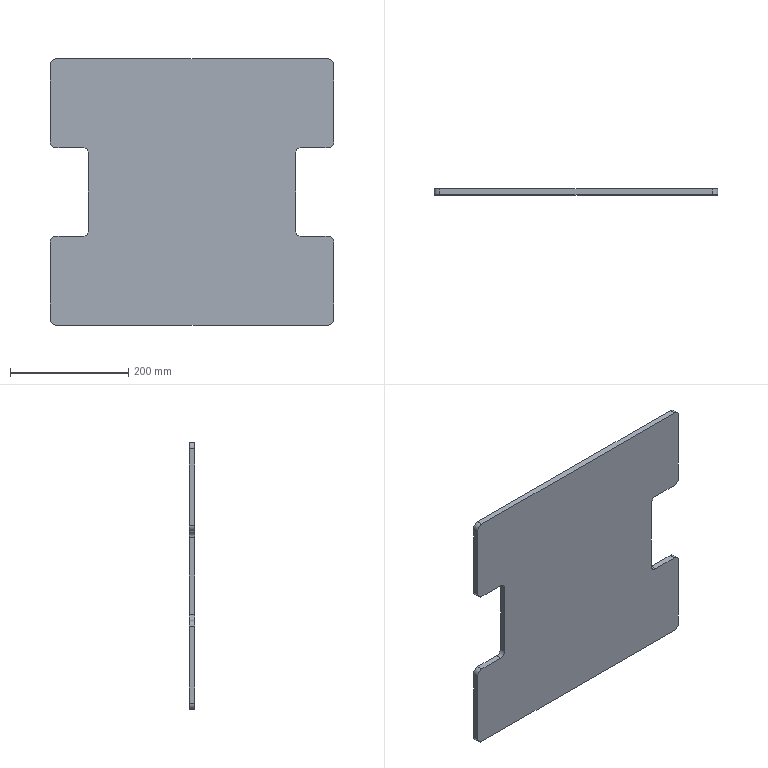Part | SolidWorks | features Fillet 2, ICE 2, Extrusion 1 | 1 solid | 26 faces | box 480 x 10 x 450 mm | volume 1964142 mm3 | plane 14 | cylinder 12 | commonest cylinder face diameters 20 x12
STEP:
#1=CARTESIAN_POINT('',(240.,0.,215.));
#2=VERTEX_POINT('',#1);
#3=CARTESIAN_POINT('',(240.,0.,85.));
#4=VERTEX_POINT('',#3);
#5=CARTESIAN_POINT('',(240.,0.,-325.));
#6=DIRECTION('',(0.,0.,-1.));
#7=VECTOR('',#6,1000.);
#8=LINE('',#5,#7);
#9=EDGE_CURVE('',#2,#4,#8,.T.);
#10=ORIENTED_EDGE('',*,*,#9,.T.);
#11=CARTESIAN_POINT('',(240.,10.,85.));
#12=VERTEX_POINT('',#11);
#13=CARTESIAN_POINT('',(240.,10.,85.));
#14=DIRECTION('',(0.,1.,0.));
#15=VECTOR('',#14,1000.);
#16=LINE('',#13,#15);
#17=EDGE_CURVE('',#4,#12,#16,.T.);
#18=ORIENTED_EDGE('',*,*,#17,.T.);
#19=CARTESIAN_POINT('',(240.,10.,215.));
#20=VERTEX_POINT('',#19);
#21=CARTESIAN_POINT('',(240.,10.,-325.));
#22=DIRECTION('',(0.,0.,-1.));
#23=VECTOR('',#22,1000.);
#24=LINE('',#21,#23);
#25=EDGE_CURVE('',#20,#12,#24,.T.);
#26=ORIENTED_EDGE('',*,*,#25,.F.);
#27=CARTESIAN_POINT('',(240.,10.,215.));
#28=DIRECTION('',(0.,-1.,0.));
#29=VECTOR('',#28,1000.);
#30=LINE('',#27,#29);
#31=EDGE_CURVE('',#20,#2,#30,.T.);
#32=ORIENTED_EDGE('',*,*,#31,.T.);
#33=EDGE_LOOP('',(#10,#18,#26,#32));
#34=FACE_OUTER_BOUND('',#33,.T.);
#35=CARTESIAN_POINT('',(240.,10.,-325.));
#36=DIRECTION('',(-1.,0.,0.));
#37=DIRECTION('',(0.,0.,1.));
#38=AXIS2_PLACEMENT_3D('',#35,#36,#37);
#39=PLANE('',#38);
#40=ADVANCED_FACE('',(#34),#39,.F.);
#41=CARTESIAN_POINT('',(-240.,10.,-215.));
#42=VERTEX_POINT('',#41);
#43=CARTESIAN_POINT('',(-240.,10.,-85.));
#44=VERTEX_POINT('',#43);
#45=CARTESIAN_POINT('',(-240.,10.,-325.));
#46=DIRECTION('',(0.,0.,1.));
#47=VECTOR('',#46,1000.);
#48=LINE('',#45,#47);
#49=EDGE_CURVE('',#42,#44,#48,.T.);
#50=ORIENTED_EDGE('',*,*,#49,.F.);
#51=CARTESIAN_POINT('',(-240.,0.,-215.));
#52=VERTEX_POINT('',#51);
#53=CARTESIAN_POINT('',(-240.,10.,-215.));
#54=DIRECTION('',(0.,-1.,0.));
#55=VECTOR('',#54,1000.);
#56=LINE('',#53,#55);
#57=EDGE_CURVE('',#42,#52,#56,.T.);
#58=ORIENTED_EDGE('',*,*,#57,.T.);
#59=CARTESIAN_POINT('',(-240.,0.,-85.));
#60=VERTEX_POINT('',#59);
#61=CARTESIAN_POINT('',(-240.,0.,-325.));
#62=DIRECTION('',(0.,0.,1.));
#63=VECTOR('',#62,1000.);
#64=LINE('',#61,#63);
#65=EDGE_CURVE('',#52,#60,#64,.T.);
#66=ORIENTED_EDGE('',*,*,#65,.T.);
#67=CARTESIAN_POINT('',(-240.,10.,-85.));
#68=DIRECTION('',(0.,1.,0.));
#69=VECTOR('',#68,1000.);
#70=LINE('',#67,#69);
#71=EDGE_CURVE('',#60,#44,#70,.T.);
#72=ORIENTED_EDGE('',*,*,#71,.T.);
#73=EDGE_LOOP('',(#50,#58,#66,#72));
#74=FACE_OUTER_BOUND('',#73,.T.);
#75=CARTESIAN_POINT('',(-240.,10.,-325.));
#76=DIRECTION('',(1.,0.,0.));
#77=DIRECTION('',(0.,0.,-1.));
#78=AXIS2_PLACEMENT_3D('',#75,#76,#77);
#79=PLANE('',#78);
#80=ADVANCED_FACE('',(#74),#79,.F.);
#81=CARTESIAN_POINT('',(-230.,10.,-225.));
#82=VERTEX_POINT('',#81);
#83=CARTESIAN_POINT('',(230.,10.,-225.));
#84=VERTEX_POINT('',#83);
#85=CARTESIAN_POINT('',(-281.378,10.,-225.));
#86=DIRECTION('',(1.,0.,0.));
#87=VECTOR('',#86,1000.);
#88=LINE('',#85,#87);
#89=EDGE_CURVE('',#82,#84,#88,.T.);
#90=ORIENTED_EDGE('',*,*,#89,.F.);
#91=CARTESIAN_POINT('',(-230.,10.,-215.));
#92=DIRECTION('',(0.,1.,0.));
#93=DIRECTION('',(0.,0.,1.));
#94=AXIS2_PLACEMENT_3D('',#91,#92,#93);
#95=CIRCLE('',#94,10.);
#96=EDGE_CURVE('',#82,#42,#95,.T.);
#97=ORIENTED_EDGE('',*,*,#96,.T.);
#98=ORIENTED_EDGE('',*,*,#49,.T.);
#99=CARTESIAN_POINT('',(-230.,10.,-75.));
#100=VERTEX_POINT('',#99);
#101=CARTESIAN_POINT('',(-230.,10.,-85.));
#102=DIRECTION('',(0.,1.,0.));
#103=DIRECTION('',(0.,0.,1.));
#104=AXIS2_PLACEMENT_3D('',#101,#102,#103);
#105=CIRCLE('',#104,10.);
#106=EDGE_CURVE('',#44,#100,#105,.T.);
#107=ORIENTED_EDGE('',*,*,#106,.T.);
#108=CARTESIAN_POINT('',(-185.,10.,-75.));
#109=VERTEX_POINT('',#108);
#110=CARTESIAN_POINT('',(-305.,10.,-75.));
#111=DIRECTION('',(1.,0.,0.));
#112=VECTOR('',#111,1000.);
#113=LINE('',#110,#112);
#114=EDGE_CURVE('',#100,#109,#113,.T.);
#115=ORIENTED_EDGE('',*,*,#114,.T.);
#116=CARTESIAN_POINT('',(-175.,10.,-65.));
#117=VERTEX_POINT('',#116);
#118=CARTESIAN_POINT('',(-185.,10.,-65.));
#119=DIRECTION('',(0.,-1.,0.));
#120=DIRECTION('',(0.,0.,1.));
#121=AXIS2_PLACEMENT_3D('',#118,#119,#120);
#122=CIRCLE('',#121,10.);
#123=EDGE_CURVE('',#109,#117,#122,.T.);
#124=ORIENTED_EDGE('',*,*,#123,.T.);
#125=CARTESIAN_POINT('',(-175.,10.,65.));
#126=VERTEX_POINT('',#125);
#127=CARTESIAN_POINT('',(-175.,10.,-75.));
#128=DIRECTION('',(0.,0.,1.));
#129=VECTOR('',#128,1000.);
#130=LINE('',#127,#129);
#131=EDGE_CURVE('',#117,#126,#130,.T.);
#132=ORIENTED_EDGE('',*,*,#131,.T.);
#133=CARTESIAN_POINT('',(-185.,10.,75.));
#134=VERTEX_POINT('',#133);
#135=CARTESIAN_POINT('',(-185.,10.,65.));
#136=DIRECTION('',(0.,-1.,0.));
#137=DIRECTION('',(0.,0.,1.));
#138=AXIS2_PLACEMENT_3D('',#135,#136,#137);
#139=CIRCLE('',#138,10.);
#140=EDGE_CURVE('',#126,#134,#139,.T.);
#141=ORIENTED_EDGE('',*,*,#140,.T.);
#142=CARTESIAN_POINT('',(-230.,10.,75.));
#143=VERTEX_POINT('',#142);
#144=CARTESIAN_POINT('',(-305.,10.,75.));
#145=DIRECTION('',(1.,0.,0.));
#146=VECTOR('',#145,1000.);
#147=LINE('',#144,#146);
#148=EDGE_CURVE('',#143,#134,#147,.T.);
#149=ORIENTED_EDGE('',*,*,#148,.F.);
#150=CARTESIAN_POINT('',(-240.,10.,85.));
#151=VERTEX_POINT('',#150);
#152=CARTESIAN_POINT('',(-230.,10.,85.));
#153=DIRECTION('',(0.,1.,0.));
#154=DIRECTION('',(0.,0.,1.));
#155=AXIS2_PLACEMENT_3D('',#152,#153,#154);
#156=CIRCLE('',#155,10.);
#157=EDGE_CURVE('',#143,#151,#156,.T.);
#158=ORIENTED_EDGE('',*,*,#157,.T.);
#159=CARTESIAN_POINT('',(-240.,10.,215.));
#160=VERTEX_POINT('',#159);
#161=CARTESIAN_POINT('',(-240.,10.,-325.));
#162=DIRECTION('',(0.,0.,1.));
#163=VECTOR('',#162,1000.);
#164=LINE('',#161,#163);
#165=EDGE_CURVE('',#151,#160,#164,.T.);
#166=ORIENTED_EDGE('',*,*,#165,.T.);
#167=CARTESIAN_POINT('',(-230.,10.,225.));
#168=VERTEX_POINT('',#167);
#169=CARTESIAN_POINT('',(-230.,10.,215.));
#170=DIRECTION('',(0.,1.,0.));
#171=DIRECTION('',(0.,0.,1.));
#172=AXIS2_PLACEMENT_3D('',#169,#170,#171);
#173=CIRCLE('',#172,10.);
#174=EDGE_CURVE('',#160,#168,#173,.T.);
#175=ORIENTED_EDGE('',*,*,#174,.T.);
#176=CARTESIAN_POINT('',(230.,10.,225.));
#177=VERTEX_POINT('',#176);
#178=CARTESIAN_POINT('',(-281.378,10.,225.));
#179=DIRECTION('',(-1.,0.,0.));
#180=VECTOR('',#179,1000.);
#181=LINE('',#178,#180);
#182=EDGE_CURVE('',#177,#168,#181,.T.);
#183=ORIENTED_EDGE('',*,*,#182,.F.);
#184=CARTESIAN_POINT('',(230.,10.,215.));
#185=DIRECTION('',(0.,1.,0.));
#186=DIRECTION('',(0.,0.,1.));
#187=AXIS2_PLACEMENT_3D('',#184,#185,#186);
#188=CIRCLE('',#187,10.);
#189=EDGE_CURVE('',#177,#20,#188,.T.);
#190=ORIENTED_EDGE('',*,*,#189,.T.);
#191=ORIENTED_EDGE('',*,*,#25,.T.);
#192=CARTESIAN_POINT('',(230.,10.,75.));
#193=VERTEX_POINT('',#192);
#194=CARTESIAN_POINT('',(230.,10.,85.));
#195=DIRECTION('',(0.,1.,0.));
#196=DIRECTION('',(0.,0.,1.));
#197=AXIS2_PLACEMENT_3D('',#194,#195,#196);
#198=CIRCLE('',#197,10.);
#199=EDGE_CURVE('',#12,#193,#198,.T.);
#200=ORIENTED_EDGE('',*,*,#199,.T.);
#201=CARTESIAN_POINT('',(185.,10.,75.));
#202=VERTEX_POINT('',#201);
#203=CARTESIAN_POINT('',(305.,10.,75.));
#204=DIRECTION('',(-1.,0.,0.));
#205=VECTOR('',#204,1000.);
#206=LINE('',#203,#205);
#207=EDGE_CURVE('',#193,#202,#206,.T.);
#208=ORIENTED_EDGE('',*,*,#207,.T.);
#209=CARTESIAN_POINT('',(175.,10.,65.));
#210=VERTEX_POINT('',#209);
#211=CARTESIAN_POINT('',(185.,10.,65.));
#212=DIRECTION('',(0.,-1.,0.));
#213=DIRECTION('',(0.,0.,1.));
#214=AXIS2_PLACEMENT_3D('',#211,#212,#213);
#215=CIRCLE('',#214,10.);
#216=EDGE_CURVE('',#202,#210,#215,.T.);
#217=ORIENTED_EDGE('',*,*,#216,.T.);
#218=CARTESIAN_POINT('',(175.,10.,-65.));
#219=VERTEX_POINT('',#218);
#220=CARTESIAN_POINT('',(175.,10.,-75.));
#221=DIRECTION('',(0.,0.,1.));
#222=VECTOR('',#221,1000.);
#223=LINE('',#220,#222);
#224=EDGE_CURVE('',#219,#210,#223,.T.);
#225=ORIENTED_EDGE('',*,*,#224,.F.);
#226=CARTESIAN_POINT('',(185.,10.,-75.));
#227=VERTEX_POINT('',#226);
#228=CARTESIAN_POINT('',(185.,10.,-65.));
#229=DIRECTION('',(0.,-1.,0.));
#230=DIRECTION('',(0.,0.,1.));
#231=AXIS2_PLACEMENT_3D('',#228,#229,#230);
#232=CIRCLE('',#231,10.);
#233=EDGE_CURVE('',#219,#227,#232,.T.);
#234=ORIENTED_EDGE('',*,*,#233,.T.);
#235=CARTESIAN_POINT('',(230.,10.,-75.));
#236=VERTEX_POINT('',#235);
#237=CARTESIAN_POINT('',(305.,10.,-75.));
#238=DIRECTION('',(-1.,0.,0.));
#239=VECTOR('',#238,1000.);
#240=LINE('',#237,#239);
#241=EDGE_CURVE('',#236,#227,#240,.T.);
#242=ORIENTED_EDGE('',*,*,#241,.F.);
#243=CARTESIAN_POINT('',(240.,10.,-85.));
#244=VERTEX_POINT('',#243);
#245=CARTESIAN_POINT('',(230.,10.,-85.));
#246=DIRECTION('',(0.,1.,0.));
#247=DIRECTION('',(0.,0.,1.));
#248=AXIS2_PLACEMENT_3D('',#245,#246,#247);
#249=CIRCLE('',#248,10.);
#250=EDGE_CURVE('',#236,#244,#249,.T.);
#251=ORIENTED_EDGE('',*,*,#250,.T.);
#252=CARTESIAN_POINT('',(240.,10.,-215.));
#253=VERTEX_POINT('',#252);
#254=CARTESIAN_POINT('',(240.,10.,-325.));
#255=DIRECTION('',(0.,0.,-1.));
#256=VECTOR('',#255,1000.);
#257=LINE('',#254,#256);
#258=EDGE_CURVE('',#244,#253,#257,.T.);
#259=ORIENTED_EDGE('',*,*,#258,.T.);
#260=CARTESIAN_POINT('',(230.,10.,-215.));
#261=DIRECTION('',(0.,1.,0.));
#262=DIRECTION('',(0.,0.,1.));
#263=AXIS2_PLACEMENT_3D('',#260,#261,#262);
#264=CIRCLE('',#263,10.);
#265=EDGE_CURVE('',#253,#84,#264,.T.);
#266=ORIENTED_EDGE('',*,*,#265,.T.);
#267=EDGE_LOOP('',(#90,#97,#98,#107,#115,#124,#132,#141,#149,#158,#166,#175,#183,#190,#191,#200,#208,#217,#225,#234,#242,#251,#259,#266));
#268=FACE_OUTER_BOUND('',#267,.T.);
#269=CARTESIAN_POINT('',(0.,10.,0.));
#270=DIRECTION('',(0.,1.,0.));
#271=DIRECTION('',(0.,0.,1.));
#272=AXIS2_PLACEMENT_3D('',#269,#270,#271);
#273=PLANE('',#272);
#274=ADVANCED_FACE('',(#268),#273,.T.);
#275=ORIENTED_EDGE('',*,*,#65,.F.);
#276=CARTESIAN_POINT('',(-230.,0.,-225.));
#277=VERTEX_POINT('',#276);
#278=CARTESIAN_POINT('',(-230.,0.,-215.));
#279=DIRECTION('',(0.,-1.,0.));
#280=DIRECTION('',(0.,0.,1.));
#281=AXIS2_PLACEMENT_3D('',#278,#279,#280);
#282=CIRCLE('',#281,10.);
#283=EDGE_CURVE('',#52,#277,#282,.T.);
#284=ORIENTED_EDGE('',*,*,#283,.T.);
#285=CARTESIAN_POINT('',(230.,0.,-225.));
#286=VERTEX_POINT('',#285);
#287=CARTESIAN_POINT('',(-281.378,0.,-225.));
#288=DIRECTION('',(1.,0.,0.));
#289=VECTOR('',#288,1000.);
#290=LINE('',#287,#289);
#291=EDGE_CURVE('',#277,#286,#290,.T.);
#292=ORIENTED_EDGE('',*,*,#291,.T.);
#293=CARTESIAN_POINT('',(240.,0.,-215.));
#294=VERTEX_POINT('',#293);
#295=CARTESIAN_POINT('',(230.,0.,-215.));
#296=DIRECTION('',(0.,-1.,0.));
#297=DIRECTION('',(0.,0.,1.));
#298=AXIS2_PLACEMENT_3D('',#295,#296,#297);
#299=CIRCLE('',#298,10.);
#300=EDGE_CURVE('',#286,#294,#299,.T.);
#301=ORIENTED_EDGE('',*,*,#300,.T.);
#302=CARTESIAN_POINT('',(240.,0.,-85.));
#303=VERTEX_POINT('',#302);
#304=CARTESIAN_POINT('',(240.,0.,-325.));
#305=DIRECTION('',(0.,0.,-1.));
#306=VECTOR('',#305,1000.);
#307=LINE('',#304,#306);
#308=EDGE_CURVE('',#303,#294,#307,.T.);
#309=ORIENTED_EDGE('',*,*,#308,.F.);
#310=CARTESIAN_POINT('',(230.,0.,-75.));
#311=VERTEX_POINT('',#310);
#312=CARTESIAN_POINT('',(230.,0.,-85.));
#313=DIRECTION('',(0.,-1.,0.));
#314=DIRECTION('',(0.,0.,1.));
#315=AXIS2_PLACEMENT_3D('',#312,#313,#314);
#316=CIRCLE('',#315,10.);
#317=EDGE_CURVE('',#303,#311,#316,.T.);
#318=ORIENTED_EDGE('',*,*,#317,.T.);
#319=CARTESIAN_POINT('',(185.,0.,-75.));
#320=VERTEX_POINT('',#319);
#321=CARTESIAN_POINT('',(0.,0.,-75.));
#322=DIRECTION('',(-1.,0.,0.));
#323=VECTOR('',#322,1000.);
#324=LINE('',#321,#323);
#325=EDGE_CURVE('',#311,#320,#324,.T.);
#326=ORIENTED_EDGE('',*,*,#325,.T.);
#327=CARTESIAN_POINT('',(175.,0.,-65.));
#328=VERTEX_POINT('',#327);
#329=CARTESIAN_POINT('',(185.,0.,-65.));
#330=DIRECTION('',(0.,1.,0.));
#331=DIRECTION('',(0.,0.,1.));
#332=AXIS2_PLACEMENT_3D('',#329,#330,#331);
#333=CIRCLE('',#332,10.);
#334=EDGE_CURVE('',#320,#328,#333,.T.);
#335=ORIENTED_EDGE('',*,*,#334,.T.);
#336=CARTESIAN_POINT('',(175.,0.,65.));
#337=VERTEX_POINT('',#336);
#338=CARTESIAN_POINT('',(175.,0.,-75.));
#339=DIRECTION('',(0.,0.,1.));
#340=VECTOR('',#339,1000.);
#341=LINE('',#338,#340);
#342=EDGE_CURVE('',#328,#337,#341,.T.);
#343=ORIENTED_EDGE('',*,*,#342,.T.);
#344=CARTESIAN_POINT('',(185.,0.,75.));
#345=VERTEX_POINT('',#344);
#346=CARTESIAN_POINT('',(185.,0.,65.));
#347=DIRECTION('',(0.,1.,0.));
#348=DIRECTION('',(0.,0.,1.));
#349=AXIS2_PLACEMENT_3D('',#346,#347,#348);
#350=CIRCLE('',#349,10.);
#351=EDGE_CURVE('',#337,#345,#350,.T.);
#352=ORIENTED_EDGE('',*,*,#351,.T.);
#353=CARTESIAN_POINT('',(230.,0.,75.));
#354=VERTEX_POINT('',#353);
#355=CARTESIAN_POINT('',(0.,0.,75.));
#356=DIRECTION('',(-1.,0.,0.));
#357=VECTOR('',#356,1000.);
#358=LINE('',#355,#357);
#359=EDGE_CURVE('',#354,#345,#358,.T.);
#360=ORIENTED_EDGE('',*,*,#359,.F.);
#361=CARTESIAN_POINT('',(230.,0.,85.));
#362=DIRECTION('',(0.,-1.,0.));
#363=DIRECTION('',(0.,0.,1.));
#364=AXIS2_PLACEMENT_3D('',#361,#362,#363);
#365=CIRCLE('',#364,10.);
#366=EDGE_CURVE('',#354,#4,#365,.T.);
#367=ORIENTED_EDGE('',*,*,#366,.T.);
#368=ORIENTED_EDGE('',*,*,#9,.F.);
#369=CARTESIAN_POINT('',(230.,0.,225.));
#370=VERTEX_POINT('',#369);
#371=CARTESIAN_POINT('',(230.,0.,215.));
#372=DIRECTION('',(0.,-1.,0.));
#373=DIRECTION('',(0.,0.,1.));
#374=AXIS2_PLACEMENT_3D('',#371,#372,#373);
#375=CIRCLE('',#374,10.);
#376=EDGE_CURVE('',#2,#370,#375,.T.);
#377=ORIENTED_EDGE('',*,*,#376,.T.);
#378=CARTESIAN_POINT('',(-230.,0.,225.));
#379=VERTEX_POINT('',#378);
#380=CARTESIAN_POINT('',(-281.378,0.,225.));
#381=DIRECTION('',(-1.,0.,0.));
#382=VECTOR('',#381,1000.);
#383=LINE('',#380,#382);
#384=EDGE_CURVE('',#370,#379,#383,.T.);
#385=ORIENTED_EDGE('',*,*,#384,.T.);
#386=CARTESIAN_POINT('',(-240.,0.,215.));
#387=VERTEX_POINT('',#386);
#388=CARTESIAN_POINT('',(-230.,0.,215.));
#389=DIRECTION('',(0.,-1.,0.));
#390=DIRECTION('',(0.,0.,1.));
#391=AXIS2_PLACEMENT_3D('',#388,#389,#390);
#392=CIRCLE('',#391,10.);
#393=EDGE_CURVE('',#379,#387,#392,.T.);
#394=ORIENTED_EDGE('',*,*,#393,.T.);
#395=CARTESIAN_POINT('',(-240.,0.,85.));
#396=VERTEX_POINT('',#395);
#397=CARTESIAN_POINT('',(-240.,0.,-325.));
#398=DIRECTION('',(0.,0.,1.));
#399=VECTOR('',#398,1000.);
#400=LINE('',#397,#399);
#401=EDGE_CURVE('',#396,#387,#400,.T.);
#402=ORIENTED_EDGE('',*,*,#401,.F.);
#403=CARTESIAN_POINT('',(-230.,0.,75.));
#404=VERTEX_POINT('',#403);
#405=CARTESIAN_POINT('',(-230.,0.,85.));
#406=DIRECTION('',(0.,-1.,0.));
#407=DIRECTION('',(0.,0.,1.));
#408=AXIS2_PLACEMENT_3D('',#405,#406,#407);
#409=CIRCLE('',#408,10.);
#410=EDGE_CURVE('',#396,#404,#409,.T.);
#411=ORIENTED_EDGE('',*,*,#410,.T.);
#412=CARTESIAN_POINT('',(-185.,0.,75.));
#413=VERTEX_POINT('',#412);
#414=CARTESIAN_POINT('',(0.,0.,75.));
#415=DIRECTION('',(1.,0.,0.));
#416=VECTOR('',#415,1000.);
#417=LINE('',#414,#416);
#418=EDGE_CURVE('',#404,#413,#417,.T.);
#419=ORIENTED_EDGE('',*,*,#418,.T.);
#420=CARTESIAN_POINT('',(-175.,0.,65.));
#421=VERTEX_POINT('',#420);
#422=CARTESIAN_POINT('',(-185.,0.,65.));
#423=DIRECTION('',(0.,1.,0.));
#424=DIRECTION('',(0.,0.,1.));
#425=AXIS2_PLACEMENT_3D('',#422,#423,#424);
#426=CIRCLE('',#425,10.);
#427=EDGE_CURVE('',#413,#421,#426,.T.);
#428=ORIENTED_EDGE('',*,*,#427,.T.);
#429=CARTESIAN_POINT('',(-175.,0.,-65.));
#430=VERTEX_POINT('',#429);
#431=CARTESIAN_POINT('',(-175.,0.,-75.));
#432=DIRECTION('',(0.,0.,1.));
#433=VECTOR('',#432,1000.);
#434=LINE('',#431,#433);
#435=EDGE_CURVE('',#430,#421,#434,.T.);
#436=ORIENTED_EDGE('',*,*,#435,.F.);
#437=CARTESIAN_POINT('',(-185.,0.,-75.));
#438=VERTEX_POINT('',#437);
#439=CARTESIAN_POINT('',(-185.,0.,-65.));
#440=DIRECTION('',(0.,1.,0.));
#441=DIRECTION('',(0.,0.,1.));
#442=AXIS2_PLACEMENT_3D('',#439,#440,#441);
#443=CIRCLE('',#442,10.);
#444=EDGE_CURVE('',#430,#438,#443,.T.);
#445=ORIENTED_EDGE('',*,*,#444,.T.);
#446=CARTESIAN_POINT('',(-230.,0.,-75.));
#447=VERTEX_POINT('',#446);
#448=CARTESIAN_POINT('',(0.,0.,-75.));
#449=DIRECTION('',(1.,0.,0.));
#450=VECTOR('',#449,1000.);
#451=LINE('',#448,#450);
#452=EDGE_CURVE('',#447,#438,#451,.T.);
#453=ORIENTED_EDGE('',*,*,#452,.F.);
#454=CARTESIAN_POINT('',(-230.,0.,-85.));
#455=DIRECTION('',(0.,-1.,0.));
#456=DIRECTION('',(0.,0.,1.));
#457=AXIS2_PLACEMENT_3D('',#454,#455,#456);
#458=CIRCLE('',#457,10.);
#459=EDGE_CURVE('',#447,#60,#458,.T.);
#460=ORIENTED_EDGE('',*,*,#459,.T.);
#461=EDGE_LOOP('',(#275,#284,#292,#301,#309,#318,#326,#335,#343,#352,#360,#367,#368,#377,#385,#394,#402,#411,#419,#428,#436,#445,#453,#460));
#462=FACE_OUTER_BOUND('',#461,.T.);
#463=CARTESIAN_POINT('',(0.,0.,0.));
#464=DIRECTION('',(0.,1.,0.));
#465=DIRECTION('',(0.,0.,1.));
#466=AXIS2_PLACEMENT_3D('',#463,#464,#465);
#467=PLANE('',#466);
#468=ADVANCED_FACE('',(#462),#467,.F.);
#469=ORIENTED_EDGE('',*,*,#308,.T.);
#470=CARTESIAN_POINT('',(240.,10.,-215.));
#471=DIRECTION('',(0.,1.,0.));
#472=VECTOR('',#471,1000.);
#473=LINE('',#470,#472);
#474=EDGE_CURVE('',#294,#253,#473,.T.);
#475=ORIENTED_EDGE('',*,*,#474,.T.);
#476=ORIENTED_EDGE('',*,*,#258,.F.);
#477=CARTESIAN_POINT('',(240.,10.,-85.));
#478=DIRECTION('',(0.,-1.,0.));
#479=VECTOR('',#478,1000.);
#480=LINE('',#477,#479);
#481=EDGE_CURVE('',#244,#303,#480,.T.);
#482=ORIENTED_EDGE('',*,*,#481,.T.);
#483=EDGE_LOOP('',(#469,#475,#476,#482));
#484=FACE_OUTER_BOUND('',#483,.T.);
#485=CARTESIAN_POINT('',(240.,10.,-325.));
#486=DIRECTION('',(-1.,0.,0.));
#487=DIRECTION('',(0.,0.,1.));
#488=AXIS2_PLACEMENT_3D('',#485,#486,#487);
#489=PLANE('',#488);
#490=ADVANCED_FACE('',(#484),#489,.F.);
#491=ORIENTED_EDGE('',*,*,#401,.T.);
#492=CARTESIAN_POINT('',(-240.,10.,215.));
#493=DIRECTION('',(0.,1.,0.));
#494=VECTOR('',#493,1000.);
#495=LINE('',#492,#494);
#496=EDGE_CURVE('',#387,#160,#495,.T.);
#497=ORIENTED_EDGE('',*,*,#496,.T.);
#498=ORIENTED_EDGE('',*,*,#165,.F.);
#499=CARTESIAN_POINT('',(-240.,10.,85.));
#500=DIRECTION('',(0.,-1.,0.));
#501=VECTOR('',#500,1000.);
#502=LINE('',#499,#501);
#503=EDGE_CURVE('',#151,#396,#502,.T.);
#504=ORIENTED_EDGE('',*,*,#503,.T.);
#505=EDGE_LOOP('',(#491,#497,#498,#504));
#506=FACE_OUTER_BOUND('',#505,.T.);
#507=CARTESIAN_POINT('',(-240.,10.,-325.));
#508=DIRECTION('',(1.,0.,0.));
#509=DIRECTION('',(0.,0.,-1.));
#510=AXIS2_PLACEMENT_3D('',#507,#508,#509);
#511=PLANE('',#510);
#512=ADVANCED_FACE('',(#506),#511,.F.);
#513=ORIENTED_EDGE('',*,*,#325,.F.);
#514=CARTESIAN_POINT('',(230.,0.,-75.));
#515=DIRECTION('',(0.,1.,0.));
#516=VECTOR('',#515,1000.);
#517=LINE('',#514,#516);
#518=EDGE_CURVE('',#311,#236,#517,.T.);
#519=ORIENTED_EDGE('',*,*,#518,.T.);
#520=ORIENTED_EDGE('',*,*,#241,.T.);
#521=CARTESIAN_POINT('',(185.,0.,-75.));
#522=DIRECTION('',(0.,-1.,0.));
#523=VECTOR('',#522,1000.);
#524=LINE('',#521,#523);
#525=EDGE_CURVE('',#227,#320,#524,.T.);
#526=ORIENTED_EDGE('',*,*,#525,.T.);
#527=EDGE_LOOP('',(#513,#519,#520,#526));
#528=FACE_OUTER_BOUND('',#527,.T.);
#529=CARTESIAN_POINT('',(305.,0.,-75.));
#530=DIRECTION('',(0.,0.,-1.));
#531=DIRECTION('',(-1.,0.,0.));
#532=AXIS2_PLACEMENT_3D('',#529,#530,#531);
#533=PLANE('',#532);
#534=ADVANCED_FACE('',(#528),#533,.F.);
#535=ORIENTED_EDGE('',*,*,#359,.T.);
#536=CARTESIAN_POINT('',(185.,0.,75.));
#537=DIRECTION('',(0.,1.,0.));
#538=VECTOR('',#537,1000.);
#539=LINE('',#536,#538);
#540=EDGE_CURVE('',#345,#202,#539,.T.);
#541=ORIENTED_EDGE('',*,*,#540,.T.);
#542=ORIENTED_EDGE('',*,*,#207,.F.);
#543=CARTESIAN_POINT('',(230.,0.,75.));
#544=DIRECTION('',(0.,-1.,0.));
#545=VECTOR('',#544,1000.);
#546=LINE('',#543,#545);
#547=EDGE_CURVE('',#193,#354,#546,.T.);
#548=ORIENTED_EDGE('',*,*,#547,.T.);
#549=EDGE_LOOP('',(#535,#541,#542,#548));
#550=FACE_OUTER_BOUND('',#549,.T.);
#551=CARTESIAN_POINT('',(305.,0.,75.));
#552=DIRECTION('',(0.,0.,-1.));
#553=DIRECTION('',(-1.,0.,0.));
#554=AXIS2_PLACEMENT_3D('',#551,#552,#553);
#555=PLANE('',#554);
#556=ADVANCED_FACE('',(#550),#555,.T.);
#557=ORIENTED_EDGE('',*,*,#342,.F.);
#558=CARTESIAN_POINT('',(175.,10.,-65.));
#559=DIRECTION('',(0.,1.,0.));
#560=VECTOR('',#559,1000.);
#561=LINE('',#558,#560);
#562=EDGE_CURVE('',#328,#219,#561,.T.);
#563=ORIENTED_EDGE('',*,*,#562,.T.);
#564=ORIENTED_EDGE('',*,*,#224,.T.);
#565=CARTESIAN_POINT('',(175.,0.,65.));
#566=DIRECTION('',(0.,-1.,0.));
#567=VECTOR('',#566,1000.);
#568=LINE('',#565,#567);
#569=EDGE_CURVE('',#210,#337,#568,.T.);
#570=ORIENTED_EDGE('',*,*,#569,.T.);
#571=EDGE_LOOP('',(#557,#563,#564,#570));
#572=FACE_OUTER_BOUND('',#571,.T.);
#573=CARTESIAN_POINT('',(175.,0.,-75.));
#574=DIRECTION('',(-1.,0.,0.));
#575=DIRECTION('',(0.,0.,1.));
#576=AXIS2_PLACEMENT_3D('',#573,#574,#575);
#577=PLANE('',#576);
#578=ADVANCED_FACE('',(#572),#577,.F.);
#579=ORIENTED_EDGE('',*,*,#452,.T.);
#580=CARTESIAN_POINT('',(-185.,10.,-75.));
#581=DIRECTION('',(0.,1.,0.));
#582=VECTOR('',#581,1000.);
#583=LINE('',#580,#582);
#584=EDGE_CURVE('',#438,#109,#583,.T.);
#585=ORIENTED_EDGE('',*,*,#584,.T.);
#586=ORIENTED_EDGE('',*,*,#114,.F.);
#587=CARTESIAN_POINT('',(-230.,0.,-75.));
#588=DIRECTION('',(0.,-1.,0.));
#589=VECTOR('',#588,1000.);
#590=LINE('',#587,#589);
#591=EDGE_CURVE('',#100,#447,#590,.T.);
#592=ORIENTED_EDGE('',*,*,#591,.T.);
#593=EDGE_LOOP('',(#579,#585,#586,#592));
#594=FACE_OUTER_BOUND('',#593,.T.);
#595=CARTESIAN_POINT('',(-305.,0.,-75.));
#596=DIRECTION('',(0.,0.,1.));
#597=DIRECTION('',(1.,0.,0.));
#598=AXIS2_PLACEMENT_3D('',#595,#596,#597);
#599=PLANE('',#598);
#600=ADVANCED_FACE('',(#594),#599,.T.);
#601=ORIENTED_EDGE('',*,*,#418,.F.);
#602=CARTESIAN_POINT('',(-230.,0.,75.));
#603=DIRECTION('',(0.,1.,0.));
#604=VECTOR('',#603,1000.);
#605=LINE('',#602,#604);
#606=EDGE_CURVE('',#404,#143,#605,.T.);
#607=ORIENTED_EDGE('',*,*,#606,.T.);
#608=ORIENTED_EDGE('',*,*,#148,.T.);
#609=CARTESIAN_POINT('',(-185.,0.,75.));
#610=DIRECTION('',(0.,-1.,0.));
#611=VECTOR('',#610,1000.);
#612=LINE('',#609,#611);
#613=EDGE_CURVE('',#134,#413,#612,.T.);
#614=ORIENTED_EDGE('',*,*,#613,.T.);
#615=EDGE_LOOP('',(#601,#607,#608,#614));
#616=FACE_OUTER_BOUND('',#615,.T.);
#617=CARTESIAN_POINT('',(-305.,0.,75.));
#618=DIRECTION('',(0.,0.,1.));
#619=DIRECTION('',(1.,0.,0.));
#620=AXIS2_PLACEMENT_3D('',#617,#618,#619);
#621=PLANE('',#620);
#622=ADVANCED_FACE('',(#616),#621,.F.);
#623=ORIENTED_EDGE('',*,*,#435,.T.);
#624=CARTESIAN_POINT('',(-175.,0.,65.));
#625=DIRECTION('',(0.,1.,0.));
#626=VECTOR('',#625,1000.);
#627=LINE('',#624,#626);
#628=EDGE_CURVE('',#421,#126,#627,.T.);
#629=ORIENTED_EDGE('',*,*,#628,.T.);
#630=ORIENTED_EDGE('',*,*,#131,.F.);
#631=CARTESIAN_POINT('',(-175.,0.,-65.));
#632=DIRECTION('',(0.,-1.,0.));
#633=VECTOR('',#632,1000.);
#634=LINE('',#631,#633);
#635=EDGE_CURVE('',#117,#430,#634,.T.);
#636=ORIENTED_EDGE('',*,*,#635,.T.);
#637=EDGE_LOOP('',(#623,#629,#630,#636));
#638=FACE_OUTER_BOUND('',#637,.T.);
#639=CARTESIAN_POINT('',(-175.,0.,-75.));
#640=DIRECTION('',(-1.,0.,0.));
#641=DIRECTION('',(0.,0.,1.));
#642=AXIS2_PLACEMENT_3D('',#639,#640,#641);
#643=PLANE('',#642);
#644=ADVANCED_FACE('',(#638),#643,.T.);
#645=ORIENTED_EDGE('',*,*,#384,.F.);
#646=CARTESIAN_POINT('',(230.,0.,225.));
#647=DIRECTION('',(0.,1.,0.));
#648=VECTOR('',#647,1000.);
#649=LINE('',#646,#648);
#650=EDGE_CURVE('',#370,#177,#649,.T.);
#651=ORIENTED_EDGE('',*,*,#650,.T.);
#652=ORIENTED_EDGE('',*,*,#182,.T.);
#653=CARTESIAN_POINT('',(-230.,0.,225.));
#654=DIRECTION('',(0.,-1.,0.));
#655=VECTOR('',#654,1000.);
#656=LINE('',#653,#655);
#657=EDGE_CURVE('',#168,#379,#656,.T.);
#658=ORIENTED_EDGE('',*,*,#657,.T.);
#659=EDGE_LOOP('',(#645,#651,#652,#658));
#660=FACE_OUTER_BOUND('',#659,.T.);
#661=CARTESIAN_POINT('',(-281.378,0.,225.));
#662=DIRECTION('',(0.,0.,-1.));
#663=DIRECTION('',(-1.,0.,0.));
#664=AXIS2_PLACEMENT_3D('',#661,#662,#663);
#665=PLANE('',#664);
#666=ADVANCED_FACE('',(#660),#665,.F.);
#667=ORIENTED_EDGE('',*,*,#291,.F.);
#668=CARTESIAN_POINT('',(-230.,0.,-225.));
#669=DIRECTION('',(0.,1.,0.));
#670=VECTOR('',#669,1000.);
#671=LINE('',#668,#670);
#672=EDGE_CURVE('',#277,#82,#671,.T.);
#673=ORIENTED_EDGE('',*,*,#672,.T.);
#674=ORIENTED_EDGE('',*,*,#89,.T.);
#675=CARTESIAN_POINT('',(230.,0.,-225.));
#676=DIRECTION('',(0.,-1.,0.));
#677=VECTOR('',#676,1000.);
#678=LINE('',#675,#677);
#679=EDGE_CURVE('',#84,#286,#678,.T.);
#680=ORIENTED_EDGE('',*,*,#679,.T.);
#681=EDGE_LOOP('',(#667,#673,#674,#680));
#682=FACE_OUTER_BOUND('',#681,.T.);
#683=CARTESIAN_POINT('',(-281.378,0.,-225.));
#684=DIRECTION('',(0.,0.,1.));
#685=DIRECTION('',(1.,0.,0.));
#686=AXIS2_PLACEMENT_3D('',#683,#684,#685);
#687=PLANE('',#686);
#688=ADVANCED_FACE('',(#682),#687,.F.);
#689=ORIENTED_EDGE('',*,*,#96,.F.);
#690=ORIENTED_EDGE('',*,*,#672,.F.);
#691=ORIENTED_EDGE('',*,*,#283,.F.);
#692=ORIENTED_EDGE('',*,*,#57,.F.);
#693=EDGE_LOOP('',(#689,#690,#691,#692));
#694=FACE_OUTER_BOUND('',#693,.T.);
#695=CARTESIAN_POINT('',(-230.,10.,-215.));
#696=DIRECTION('',(0.,-1.,0.));
#697=DIRECTION('',(0.,0.,-1.));
#698=AXIS2_PLACEMENT_3D('',#695,#696,#697);
#699=CYLINDRICAL_SURFACE('',#698,10.);
#700=ADVANCED_FACE('',(#694),#699,.T.);
#701=ORIENTED_EDGE('',*,*,#300,.F.);
#702=ORIENTED_EDGE('',*,*,#679,.F.);
#703=ORIENTED_EDGE('',*,*,#265,.F.);
#704=ORIENTED_EDGE('',*,*,#474,.F.);
#705=EDGE_LOOP('',(#701,#702,#703,#704));
#706=FACE_OUTER_BOUND('',#705,.T.);
#707=CARTESIAN_POINT('',(230.,10.,-215.));
#708=DIRECTION('',(0.,1.,0.));
#709=DIRECTION('',(0.,0.,1.));
#710=AXIS2_PLACEMENT_3D('',#707,#708,#709);
#711=CYLINDRICAL_SURFACE('',#710,10.);
#712=ADVANCED_FACE('',(#706),#711,.T.);
#713=ORIENTED_EDGE('',*,*,#250,.F.);
#714=ORIENTED_EDGE('',*,*,#518,.F.);
#715=ORIENTED_EDGE('',*,*,#317,.F.);
#716=ORIENTED_EDGE('',*,*,#481,.F.);
#717=EDGE_LOOP('',(#713,#714,#715,#716));
#718=FACE_OUTER_BOUND('',#717,.T.);
#719=CARTESIAN_POINT('',(230.,10.,-85.));
#720=DIRECTION('',(0.,-1.,0.));
#721=DIRECTION('',(0.,0.,-1.));
#722=AXIS2_PLACEMENT_3D('',#719,#720,#721);
#723=CYLINDRICAL_SURFACE('',#722,10.);
#724=ADVANCED_FACE('',(#718),#723,.T.);
#725=ORIENTED_EDGE('',*,*,#334,.F.);
#726=ORIENTED_EDGE('',*,*,#525,.F.);
#727=ORIENTED_EDGE('',*,*,#233,.F.);
#728=ORIENTED_EDGE('',*,*,#562,.F.);
#729=EDGE_LOOP('',(#725,#726,#727,#728));
#730=FACE_OUTER_BOUND('',#729,.T.);
#731=CARTESIAN_POINT('',(185.,0.,-65.));
#732=DIRECTION('',(0.,-1.,0.));
#733=DIRECTION('',(0.,0.,-1.));
#734=AXIS2_PLACEMENT_3D('',#731,#732,#733);
#735=CYLINDRICAL_SURFACE('',#734,10.);
#736=ADVANCED_FACE('',(#730),#735,.F.);
#737=ORIENTED_EDGE('',*,*,#351,.F.);
#738=ORIENTED_EDGE('',*,*,#569,.F.);
#739=ORIENTED_EDGE('',*,*,#216,.F.);
#740=ORIENTED_EDGE('',*,*,#540,.F.);
#741=EDGE_LOOP('',(#737,#738,#739,#740));
#742=FACE_OUTER_BOUND('',#741,.T.);
#743=CARTESIAN_POINT('',(185.,0.,65.));
#744=DIRECTION('',(0.,1.,0.));
#745=DIRECTION('',(0.,0.,1.));
#746=AXIS2_PLACEMENT_3D('',#743,#744,#745);
#747=CYLINDRICAL_SURFACE('',#746,10.);
#748=ADVANCED_FACE('',(#742),#747,.F.);
#749=ORIENTED_EDGE('',*,*,#199,.F.);
#750=ORIENTED_EDGE('',*,*,#17,.F.);
#751=ORIENTED_EDGE('',*,*,#366,.F.);
#752=ORIENTED_EDGE('',*,*,#547,.F.);
#753=EDGE_LOOP('',(#749,#750,#751,#752));
#754=FACE_OUTER_BOUND('',#753,.T.);
#755=CARTESIAN_POINT('',(230.,0.,85.));
#756=DIRECTION('',(0.,1.,0.));
#757=DIRECTION('',(0.,0.,1.));
#758=AXIS2_PLACEMENT_3D('',#755,#756,#757);
#759=CYLINDRICAL_SURFACE('',#758,10.);
#760=ADVANCED_FACE('',(#754),#759,.T.);
#761=ORIENTED_EDGE('',*,*,#189,.F.);
#762=ORIENTED_EDGE('',*,*,#650,.F.);
#763=ORIENTED_EDGE('',*,*,#376,.F.);
#764=ORIENTED_EDGE('',*,*,#31,.F.);
#765=EDGE_LOOP('',(#761,#762,#763,#764));
#766=FACE_OUTER_BOUND('',#765,.T.);
#767=CARTESIAN_POINT('',(230.,10.,215.));
#768=DIRECTION('',(0.,-1.,0.));
#769=DIRECTION('',(0.,0.,-1.));
#770=AXIS2_PLACEMENT_3D('',#767,#768,#769);
#771=CYLINDRICAL_SURFACE('',#770,10.);
#772=ADVANCED_FACE('',(#766),#771,.T.);
#773=ORIENTED_EDGE('',*,*,#393,.F.);
#774=ORIENTED_EDGE('',*,*,#657,.F.);
#775=ORIENTED_EDGE('',*,*,#174,.F.);
#776=ORIENTED_EDGE('',*,*,#496,.F.);
#777=EDGE_LOOP('',(#773,#774,#775,#776));
#778=FACE_OUTER_BOUND('',#777,.T.);
#779=CARTESIAN_POINT('',(-230.,10.,215.));
#780=DIRECTION('',(0.,1.,0.));
#781=DIRECTION('',(0.,0.,1.));
#782=AXIS2_PLACEMENT_3D('',#779,#780,#781);
#783=CYLINDRICAL_SURFACE('',#782,10.);
#784=ADVANCED_FACE('',(#778),#783,.T.);
#785=ORIENTED_EDGE('',*,*,#157,.F.);
#786=ORIENTED_EDGE('',*,*,#606,.F.);
#787=ORIENTED_EDGE('',*,*,#410,.F.);
#788=ORIENTED_EDGE('',*,*,#503,.F.);
#789=EDGE_LOOP('',(#785,#786,#787,#788));
#790=FACE_OUTER_BOUND('',#789,.T.);
#791=CARTESIAN_POINT('',(-230.,10.,85.));
#792=DIRECTION('',(0.,-1.,0.));
#793=DIRECTION('',(0.,0.,-1.));
#794=AXIS2_PLACEMENT_3D('',#791,#792,#793);
#795=CYLINDRICAL_SURFACE('',#794,10.);
#796=ADVANCED_FACE('',(#790),#795,.T.);
#797=ORIENTED_EDGE('',*,*,#427,.F.);
#798=ORIENTED_EDGE('',*,*,#613,.F.);
#799=ORIENTED_EDGE('',*,*,#140,.F.);
#800=ORIENTED_EDGE('',*,*,#628,.F.);
#801=EDGE_LOOP('',(#797,#798,#799,#800));
#802=FACE_OUTER_BOUND('',#801,.T.);
#803=CARTESIAN_POINT('',(-185.,0.,65.));
#804=DIRECTION('',(0.,1.,0.));
#805=DIRECTION('',(0.,0.,1.));
#806=AXIS2_PLACEMENT_3D('',#803,#804,#805);
#807=CYLINDRICAL_SURFACE('',#806,10.);
#808=ADVANCED_FACE('',(#802),#807,.F.);
#809=ORIENTED_EDGE('',*,*,#444,.F.);
#810=ORIENTED_EDGE('',*,*,#635,.F.);
#811=ORIENTED_EDGE('',*,*,#123,.F.);
#812=ORIENTED_EDGE('',*,*,#584,.F.);
#813=EDGE_LOOP('',(#809,#810,#811,#812));
#814=FACE_OUTER_BOUND('',#813,.T.);
#815=CARTESIAN_POINT('',(-185.,0.,-65.));
#816=DIRECTION('',(0.,-1.,0.));
#817=DIRECTION('',(0.,0.,-1.));
#818=AXIS2_PLACEMENT_3D('',#815,#816,#817);
#819=CYLINDRICAL_SURFACE('',#818,10.);
#820=ADVANCED_FACE('',(#814),#819,.F.);
#821=ORIENTED_EDGE('',*,*,#106,.F.);
#822=ORIENTED_EDGE('',*,*,#71,.F.);
#823=ORIENTED_EDGE('',*,*,#459,.F.);
#824=ORIENTED_EDGE('',*,*,#591,.F.);
#825=EDGE_LOOP('',(#821,#822,#823,#824));
#826=FACE_OUTER_BOUND('',#825,.T.);
#827=CARTESIAN_POINT('',(-230.,0.,-85.));
#828=DIRECTION('',(0.,1.,0.));
#829=DIRECTION('',(0.,0.,1.));
#830=AXIS2_PLACEMENT_3D('',#827,#828,#829);
#831=CYLINDRICAL_SURFACE('',#830,10.);
#832=ADVANCED_FACE('',(#826),#831,.T.);
#833=CLOSED_SHELL('',(#40,#80,#274,#468,#490,#512,#534,#556,#578,#600,#622,#644,#666,#688,#700,#712,#724,#736,#748,#760,#772,#784,#796,#808,#820,#832));
#834=MANIFOLD_SOLID_BREP('',#833);
#835=CARTESIAN_POINT('',(0.,0.,0.));
#836=DIRECTION('',(0.,0.,1.));
#837=DIRECTION('',(1.,0.,0.));
#838=AXIS2_PLACEMENT_3D('',#835,#836,#837);
#839=(LENGTH_UNIT()NAMED_UNIT(*)SI_UNIT(.MILLI.,.METRE.));
#840=UNCERTAINTY_MEASURE_WITH_UNIT(LENGTH_MEASURE(0.00001),#839,'','');
#841=(NAMED_UNIT(*)PLANE_ANGLE_UNIT()SI_UNIT($,.RADIAN.));
#842=(NAMED_UNIT(*)SI_UNIT($,.STERADIAN.)SOLID_ANGLE_UNIT());
#843=(GEOMETRIC_REPRESENTATION_CONTEXT(3)GLOBAL_UNCERTAINTY_ASSIGNED_CONTEXT((#840))GLOBAL_UNIT_ASSIGNED_CONTEXT((#839,#841,#842))REPRESENTATION_CONTEXT('',''));
#844=ADVANCED_BREP_SHAPE_REPRESENTATION('',(#834,#838),#843);